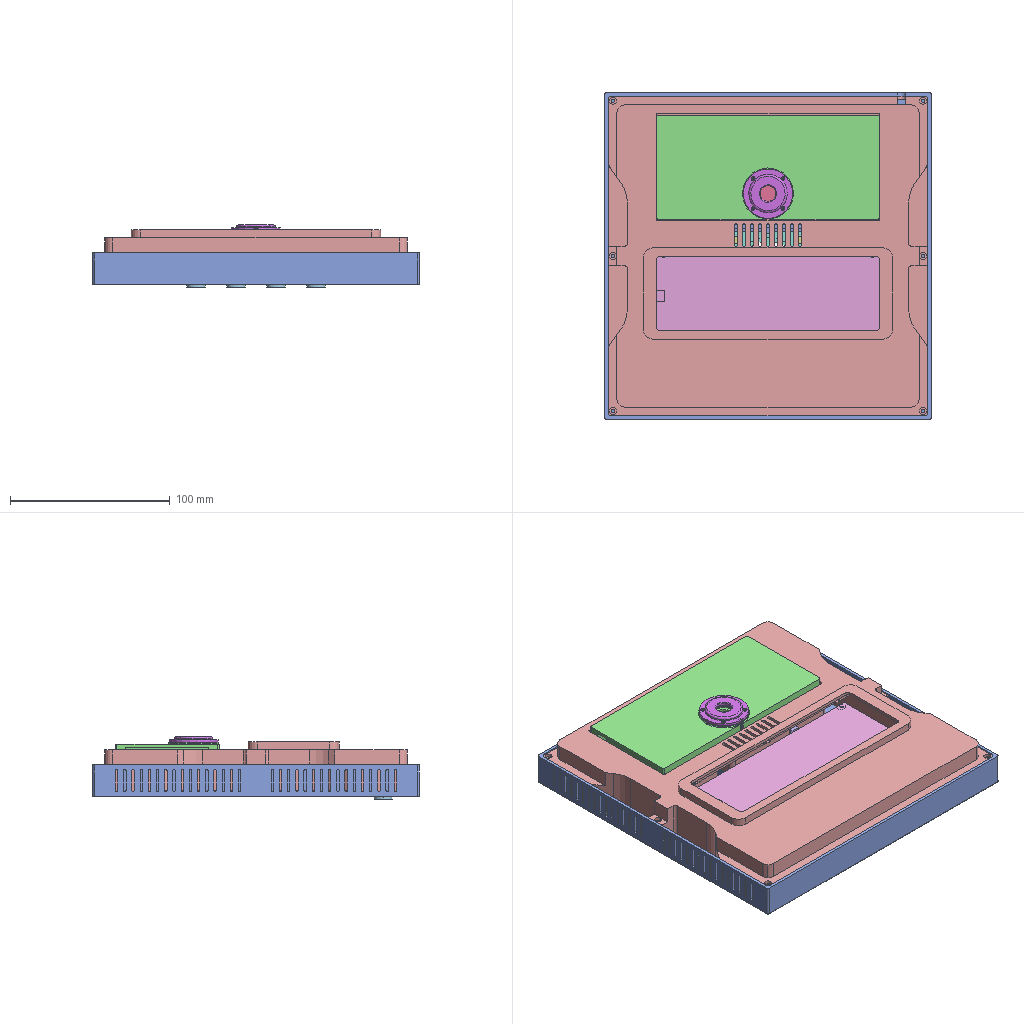Assembly | SolidWorks | 12 different items | 12 placed | box 204 x 204 x 39 mm
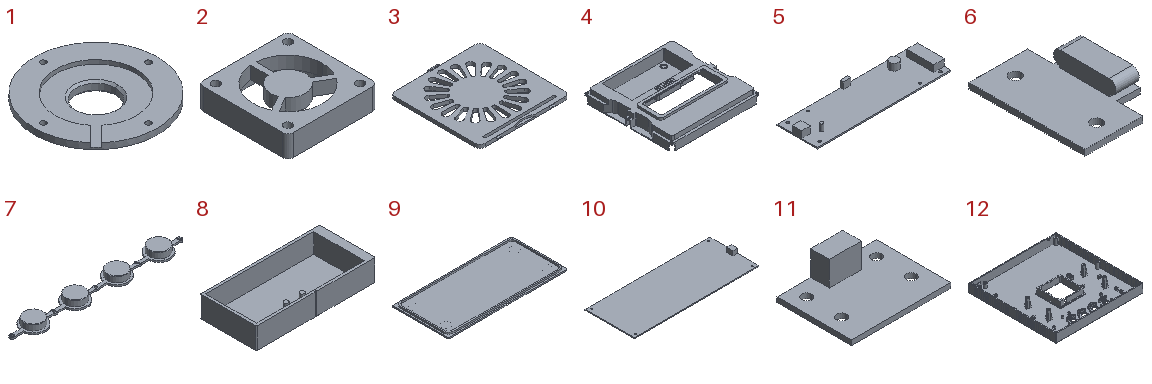Parts list (item | quantity | size | volume | features):
1 | x1 | 31 x 31 x 3.5 mm | 1459 mm3 | features ICE 5, Chamfer 1, Extrusion 1, Fillet 1
2 | x1 | 50 x 50 x 12 mm | 16391 mm3 | features ICE 2, Extrusion 1
3 | x1 | 52.5 x 54.75 x 2.2 mm | 4171 mm3 | features ICE 4, Extrusion 1, MirrorPattern 1
4 | x1 | 199.7 x 199.7 x 32.5 mm | 138569 mm3 | features ICE 30, Fillet 3, Chamfer 1, Extrusion 1, LPattern 1, Shell 1
5 | x1 | 100 x 30 x 8 mm | 4377 mm3 | features ICE 4, Extrusion 1
6 | x1 | 14 x 20 x 3.696 mm | 327.493 mm3 | features ICE 4, Extrusion 1
7 | x1 | 103 x 14 x 6.5 mm | 2303 mm3 | features Chamfer 2, ICE 2, Extrusion 1
8 | x1 | 139 x 65 x 26.2 mm | 46705 mm3 | features ICE 12, Fillet 3, Extrusion 1, Shell 1
9 | x1 | 139 x 65 x 4.5 mm | 14558 mm3 | features ICE 4, Extrusion 1
10 | x1 | 140 x 55 x 6 mm | 7876 mm3 | features Extrusion 1, ICE 1
11 | x1 | 20 x 15 x 6 mm | 407.762 mm3 | features Extrusion 1, ICE 1
12 | x1 | 204 x 204 x 24 mm | 118665 mm3 | features ICE 31, Fillet 5, Chamfer 3, Extrusion 1, MirrorPattern 1, Shell 1
Mates (type | each side: item.copy, entity, surface, feature):
Parallel | 4.1 face plane Boss-Extrude2 | 12.1 face plane Boss-Extrude1
Coincident | 4.1 face plane Boss-Extrude1 | 12.1 face plane Shell1
DistanceDim | 5.1 face plane Boss-Extrude1 | 12.1 face plane Boss-Extrude1
DistanceDim | 10.1 face plane Boss-Extrude1 | 4.1 face plane Shell1
DistanceDim | 2.1 face plane Boss-Extrude1 | 12.1 face plane Cut-Extrude1 | 2 times
DistanceDim | 6.1 face plane Boss-Extrude1 | 4.1 face plane Boss-Extrude1
DistanceDim | 2.1 face plane Boss-Extrude1 | 12.1 face plane Cut-Extrude4
DistanceDim | 4.1 face plane Shell1 | 10.1 face plane Boss-Extrude1
Coincident | 12.1 face plane Boss-Extrude5 | 5.1 face plane Boss-Extrude1
DistanceDim | 11.1 face plane Boss-Extrude1 | 12.1 face plane Shell1
Coincident | 8.1 face plane Boss-Extrude1 | 9.1 face plane Boss-Extrude1 | 4 times
DistanceDim | 8.1 face plane Boss-Extrude1 | 4.1 face plane Cut-Extrude3 | 2 times
Concentric | 12.1 face cylinder Cut-Extrude1 | 7.1 face cylinder Boss-Extrude2 | 2 times
Coincident | 12.1 face plane Shell1 | 7.1 face plane Boss-Extrude1
DistanceDim | 3.1 face plane Boss-Extrude1 | 12.1 face plane Cut-Extrude4 | 2 times
Coincident | 12.1 face plane Boss-Extrude1 | 3.1 face plane Boss-Extrude1
Coincident | 4.1 face plane Boss-Extrude5 | 9.1 face plane Boss-Extrude2
Concentric | 8.1 face cylinder Cut-Extrude4 | 1.1 face cylinder Boss-Extrude2
Coincident | 1.1 face plane Boss-Extrude2 | 8.1 face plane Boss-Extrude7
Concentric | 8.1 face cylinder Cut-Extrude5 | 1.1 face cylinder Cut-Extrude2
DistanceDim | 4.1 face plane Cut-Extrude11 | 12.1 face plane Shell1 | 2 times
Concentric | 12.1 face cylinder Boss-Extrude8 | 11.1 face cylinder Boss-Extrude1 | 2 times
DistanceDim | 10.1 vertex | 4.1 face plane Boss-Extrude4